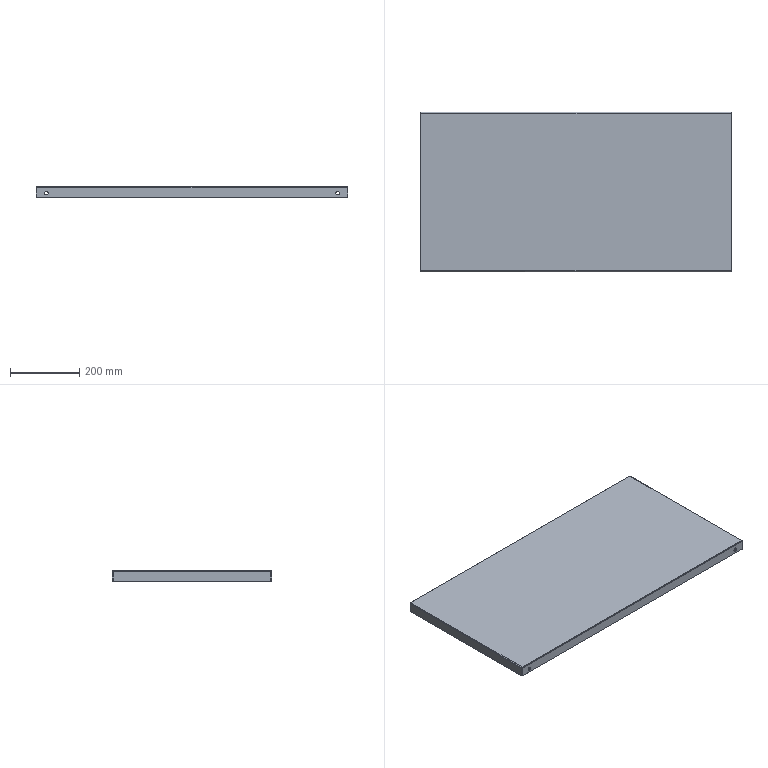Part | SolidWorks | features EdgeFlange 2, FlatPattern 1, HoleWzd 1, SMBaseFlange 1, SheetMetal 1 | 1 solid | 46 faces | box 900 x 460 x 30 mm | volume 974397 mm3 | plane 22 | cylinder 16 | spline 8 | commonest cylinder face diameters 10 x8 1.473 x4 5.473 x4